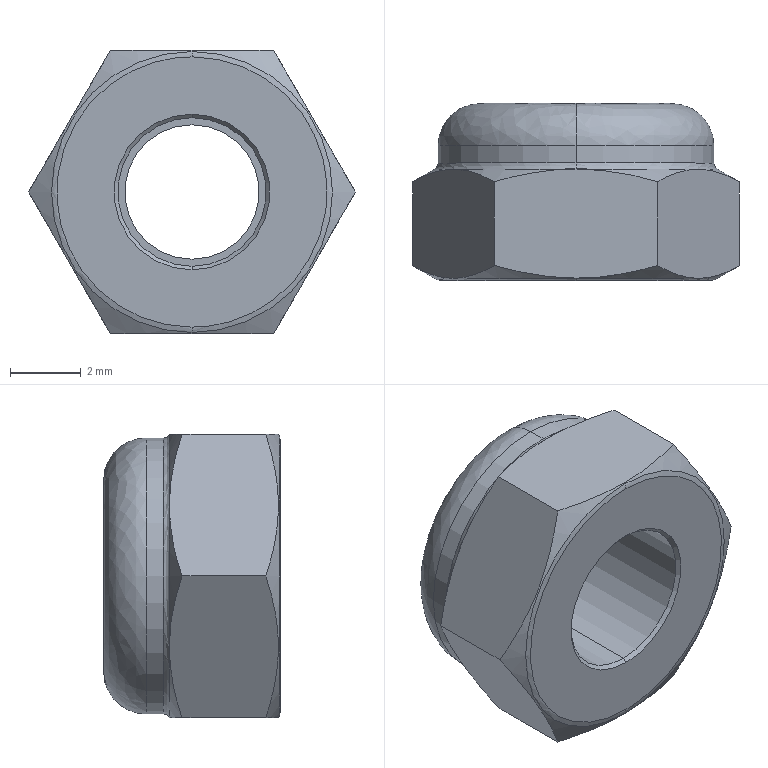Part | SolidWorks | features BaseBody 1 | 1 solid | 39 faces | box 9.238 x 5 x 8 mm | volume 186.691 mm3 | plane 11 | cone 10 | cylinder 10 | spline 8 | commonest cylinder face diameters 3.8 x2 4.2 x2 5 x2 6 x2 7.8 x2
STEP:
#1=CARTESIAN_POINT('',(0.,-1.56,3.97));
#2=VERTEX_POINT('',#1);
#3=CARTESIAN_POINT('',(0.,-1.56,-3.97));
#4=VERTEX_POINT('',#3);
#5=CARTESIAN_POINT('',(0.,-1.56,0.));
#6=DIRECTION('',(0.,-1.,0.));
#7=DIRECTION('',(0.,0.,1.));
#8=AXIS2_PLACEMENT_3D('',#5,#6,#7);
#9=CIRCLE('',#8,3.97);
#10=EDGE_CURVE('',#2,#4,#9,.T.);
#11=ORIENTED_EDGE('',*,*,#10,.T.);
#12=CARTESIAN_POINT('',(0.,-1.6,-3.82));
#13=VERTEX_POINT('',#12);
#14=CARTESIAN_POINT('',(0.,-1.3,-3.82));
#15=DIRECTION('',(-1.,0.,0.));
#16=DIRECTION('',(0.,0.,-1.));
#17=AXIS2_PLACEMENT_3D('',#14,#15,#16);
#18=CIRCLE('',#17,0.3);
#19=EDGE_CURVE('',#4,#13,#18,.T.);
#20=ORIENTED_EDGE('',*,*,#19,.T.);
#21=CARTESIAN_POINT('',(0.,-1.6,3.82));
#22=VERTEX_POINT('',#21);
#23=CARTESIAN_POINT('',(0.,-1.6,-3.82));
#24=CARTESIAN_POINT('',(-7.639,-1.6,-3.82));
#25=CARTESIAN_POINT('',(-7.639,-1.6,3.82));
#26=CARTESIAN_POINT('',(0.,-1.6,3.82));
#27=(BOUNDED_CURVE()B_SPLINE_CURVE(3,(#23,#24,#25,#26),.UNSPECIFIED.,.F.,.F.)B_SPLINE_CURVE_WITH_KNOTS((4,4),(0.,1.),.UNSPECIFIED.)CURVE()GEOMETRIC_REPRESENTATION_ITEM()RATIONAL_B_SPLINE_CURVE((1.,0.3333,0.3333,1.))REPRESENTATION_ITEM(''));
#28=EDGE_CURVE('',#13,#22,#27,.T.);
#29=ORIENTED_EDGE('',*,*,#28,.T.);
#30=CARTESIAN_POINT('',(0.,-1.3,3.82));
#31=DIRECTION('',(1.,0.,0.));
#32=DIRECTION('',(0.,0.,1.));
#33=AXIS2_PLACEMENT_3D('',#30,#31,#32);
#34=CIRCLE('',#33,0.3);
#35=EDGE_CURVE('',#2,#22,#34,.T.);
#36=ORIENTED_EDGE('',*,*,#35,.F.);
#37=EDGE_LOOP('',(#11,#20,#29,#36));
#38=FACE_OUTER_BOUND('',#37,.T.);
#39=CARTESIAN_POINT('',(0.,-1.56,-3.97));
#40=CARTESIAN_POINT('',(-7.939,-1.56,-3.97));
#41=CARTESIAN_POINT('',(-7.939,-1.56,3.97));
#42=CARTESIAN_POINT('',(0.,-1.56,3.97));
#43=CARTESIAN_POINT('',(0.,-1.586,-3.924));
#44=CARTESIAN_POINT('',(-7.847,-1.586,-3.924));
#45=CARTESIAN_POINT('',(-7.847,-1.586,3.924));
#46=CARTESIAN_POINT('',(0.,-1.586,3.924));
#47=CARTESIAN_POINT('',(0.,-1.6,-3.873));
#48=CARTESIAN_POINT('',(-7.745,-1.6,-3.873));
#49=CARTESIAN_POINT('',(-7.745,-1.6,3.873));
#50=CARTESIAN_POINT('',(0.,-1.6,3.873));
#51=CARTESIAN_POINT('',(0.,-1.6,-3.82));
#52=CARTESIAN_POINT('',(-7.639,-1.6,-3.82));
#53=CARTESIAN_POINT('',(-7.639,-1.6,3.82));
#54=CARTESIAN_POINT('',(0.,-1.6,3.82));
#55=(BOUNDED_SURFACE()B_SPLINE_SURFACE(3,3,((#39,#40,#41,#42),(#43,#44,#45,#46),(#47,#48,#49,#50),(#51,#52,#53,#54)),.UNSPECIFIED.,.F.,.F.,.F.)B_SPLINE_SURFACE_WITH_KNOTS((4,4),(4,4),(0.,1.),(0.,1.),.UNSPECIFIED.)GEOMETRIC_REPRESENTATION_ITEM()RATIONAL_B_SPLINE_SURFACE(((1.,0.3333,0.3333,1.),(0.9773,0.3258,0.3258,0.9773),(0.9773,0.3258,0.3258,0.9773),(1.,0.3333,0.3333,1.)))REPRESENTATION_ITEM('')SURFACE());
#56=ADVANCED_FACE('',(#38),#55,.T.);
#57=CARTESIAN_POINT('',(0.,1.542,-4.));
#58=VERTEX_POINT('',#57);
#59=CARTESIAN_POINT('',(3.464,1.542,-2.));
#60=VERTEX_POINT('',#59);
#61=CARTESIAN_POINT('',(0.,1.542,0.));
#62=DIRECTION('',(0.,-1.,0.));
#63=DIRECTION('',(0.,0.,-1.));
#64=AXIS2_PLACEMENT_3D('',#61,#62,#63);
#65=CIRCLE('',#64,4.);
#66=EDGE_CURVE('',#58,#60,#65,.T.);
#67=ORIENTED_EDGE('',*,*,#66,.F.);
#68=CARTESIAN_POINT('',(0.,1.715,-3.9));
#69=VERTEX_POINT('',#68);
#70=CARTESIAN_POINT('',(0.,1.715,-4.1));
#71=DIRECTION('',(-1.,0.,0.));
#72=DIRECTION('',(0.,0.,-1.));
#73=AXIS2_PLACEMENT_3D('',#70,#71,#72);
#74=CIRCLE('',#73,0.2);
#75=EDGE_CURVE('',#58,#69,#74,.T.);
#76=ORIENTED_EDGE('',*,*,#75,.T.);
#77=CARTESIAN_POINT('',(0.,1.715,3.9));
#78=VERTEX_POINT('',#77);
#79=CARTESIAN_POINT('',(0.,1.715,0.));
#80=DIRECTION('',(0.,1.,0.));
#81=DIRECTION('',(0.,0.,1.));
#82=AXIS2_PLACEMENT_3D('',#79,#80,#81);
#83=CIRCLE('',#82,3.9);
#84=EDGE_CURVE('',#78,#69,#83,.T.);
#85=ORIENTED_EDGE('',*,*,#84,.F.);
#86=CARTESIAN_POINT('',(0.,1.542,4.));
#87=VERTEX_POINT('',#86);
#88=CARTESIAN_POINT('',(0.,1.715,4.1));
#89=DIRECTION('',(1.,0.,0.));
#90=DIRECTION('',(0.,0.,1.));
#91=AXIS2_PLACEMENT_3D('',#88,#89,#90);
#92=CIRCLE('',#91,0.2);
#93=EDGE_CURVE('',#87,#78,#92,.T.);
#94=ORIENTED_EDGE('',*,*,#93,.F.);
#95=CARTESIAN_POINT('',(3.464,1.542,2.));
#96=VERTEX_POINT('',#95);
#97=CARTESIAN_POINT('',(0.,1.542,0.));
#98=DIRECTION('',(0.,-1.,0.));
#99=DIRECTION('',(0.,0.,-1.));
#100=AXIS2_PLACEMENT_3D('',#97,#98,#99);
#101=CIRCLE('',#100,4.);
#102=EDGE_CURVE('',#96,#87,#101,.T.);
#103=ORIENTED_EDGE('',*,*,#102,.F.);
#104=CARTESIAN_POINT('',(0.,1.542,0.));
#105=DIRECTION('',(0.,-1.,0.));
#106=DIRECTION('',(0.,0.,-1.));
#107=AXIS2_PLACEMENT_3D('',#104,#105,#106);
#108=CIRCLE('',#107,4.);
#109=EDGE_CURVE('',#60,#96,#108,.T.);
#110=ORIENTED_EDGE('',*,*,#109,.F.);
#111=EDGE_LOOP('',(#67,#76,#85,#94,#103,#110));
#112=FACE_OUTER_BOUND('',#111,.T.);
#113=CARTESIAN_POINT('',(0.,1.542,4.));
#114=CARTESIAN_POINT('',(8.,1.542,4.));
#115=CARTESIAN_POINT('',(8.,1.542,-4.));
#116=CARTESIAN_POINT('',(0.,1.542,-4.));
#117=CARTESIAN_POINT('',(0.,1.579,3.937));
#118=CARTESIAN_POINT('',(7.873,1.579,3.937));
#119=CARTESIAN_POINT('',(7.873,1.579,-3.937));
#120=CARTESIAN_POINT('',(0.,1.579,-3.937));
#121=CARTESIAN_POINT('',(0.,1.642,3.9));
#122=CARTESIAN_POINT('',(7.8,1.642,3.9));
#123=CARTESIAN_POINT('',(7.8,1.642,-3.9));
#124=CARTESIAN_POINT('',(0.,1.642,-3.9));
#125=CARTESIAN_POINT('',(0.,1.715,3.9));
#126=CARTESIAN_POINT('',(7.8,1.715,3.9));
#127=CARTESIAN_POINT('',(7.8,1.715,-3.9));
#128=CARTESIAN_POINT('',(0.,1.715,-3.9));
#129=(BOUNDED_SURFACE()B_SPLINE_SURFACE(3,3,((#113,#114,#115,#116),(#117,#118,#119,#120),(#121,#122,#123,#124),(#125,#126,#127,#128)),.UNSPECIFIED.,.F.,.F.,.F.)B_SPLINE_SURFACE_WITH_KNOTS((4,4),(4,4),(0.,1.),(0.,1.),.UNSPECIFIED.)GEOMETRIC_REPRESENTATION_ITEM()RATIONAL_B_SPLINE_SURFACE(((1.,0.3333,0.3333,1.),(0.9107,0.3036,0.3036,0.9107),(0.9107,0.3036,0.3036,0.9107),(1.,0.3333,0.3333,1.)))REPRESENTATION_ITEM('')SURFACE());
#130=ADVANCED_FACE('',(#112),#129,.F.);
#131=CARTESIAN_POINT('',(0.,3.4,2.7));
#132=VERTEX_POINT('',#131);
#133=CARTESIAN_POINT('',(0.,3.4,-2.7));
#134=VERTEX_POINT('',#133);
#135=CARTESIAN_POINT('',(0.,3.4,2.7));
#136=CARTESIAN_POINT('',(-5.4,3.4,2.7));
#137=CARTESIAN_POINT('',(-5.4,3.4,-2.7));
#138=CARTESIAN_POINT('',(0.,3.4,-2.7));
#139=(BOUNDED_CURVE()B_SPLINE_CURVE(3,(#135,#136,#137,#138),.UNSPECIFIED.,.F.,.F.)B_SPLINE_CURVE_WITH_KNOTS((4,4),(0.,1.),.UNSPECIFIED.)CURVE()GEOMETRIC_REPRESENTATION_ITEM()RATIONAL_B_SPLINE_CURVE((1.,0.3333,0.3333,1.))REPRESENTATION_ITEM(''));
#140=EDGE_CURVE('',#132,#134,#139,.T.);
#141=ORIENTED_EDGE('',*,*,#140,.T.);
#142=CARTESIAN_POINT('',(0.,2.2,-3.9));
#143=VERTEX_POINT('',#142);
#144=CARTESIAN_POINT('',(0.,2.2,-2.7));
#145=DIRECTION('',(-1.,0.,0.));
#146=DIRECTION('',(0.,0.,-1.));
#147=AXIS2_PLACEMENT_3D('',#144,#145,#146);
#148=CIRCLE('',#147,1.2);
#149=EDGE_CURVE('',#134,#143,#148,.T.);
#150=ORIENTED_EDGE('',*,*,#149,.T.);
#151=CARTESIAN_POINT('',(0.,2.2,3.9));
#152=VERTEX_POINT('',#151);
#153=CARTESIAN_POINT('',(0.,2.2,0.));
#154=DIRECTION('',(0.,-1.,0.));
#155=DIRECTION('',(0.,0.,1.));
#156=AXIS2_PLACEMENT_3D('',#153,#154,#155);
#157=CIRCLE('',#156,3.9);
#158=EDGE_CURVE('',#152,#143,#157,.T.);
#159=ORIENTED_EDGE('',*,*,#158,.F.);
#160=CARTESIAN_POINT('',(0.,2.2,2.7));
#161=DIRECTION('',(1.,0.,0.));
#162=DIRECTION('',(0.,0.,1.));
#163=AXIS2_PLACEMENT_3D('',#160,#161,#162);
#164=CIRCLE('',#163,1.2);
#165=EDGE_CURVE('',#132,#152,#164,.T.);
#166=ORIENTED_EDGE('',*,*,#165,.F.);
#167=EDGE_LOOP('',(#141,#150,#159,#166));
#168=FACE_OUTER_BOUND('',#167,.T.);
#169=CARTESIAN_POINT('',(0.,3.4,-2.7));
#170=CARTESIAN_POINT('',(-5.4,3.4,-2.7));
#171=CARTESIAN_POINT('',(-5.4,3.4,2.7));
#172=CARTESIAN_POINT('',(0.,3.4,2.7));
#173=CARTESIAN_POINT('',(0.,3.4,-3.403));
#174=CARTESIAN_POINT('',(-6.806,3.4,-3.403));
#175=CARTESIAN_POINT('',(-6.806,3.4,3.403));
#176=CARTESIAN_POINT('',(0.,3.4,3.403));
#177=CARTESIAN_POINT('',(0.,2.903,-3.9));
#178=CARTESIAN_POINT('',(-7.8,2.903,-3.9));
#179=CARTESIAN_POINT('',(-7.8,2.903,3.9));
#180=CARTESIAN_POINT('',(0.,2.903,3.9));
#181=CARTESIAN_POINT('',(0.,2.2,-3.9));
#182=CARTESIAN_POINT('',(-7.8,2.2,-3.9));
#183=CARTESIAN_POINT('',(-7.8,2.2,3.9));
#184=CARTESIAN_POINT('',(0.,2.2,3.9));
#185=(BOUNDED_SURFACE()B_SPLINE_SURFACE(3,3,((#169,#170,#171,#172),(#173,#174,#175,#176),(#177,#178,#179,#180),(#181,#182,#183,#184)),.UNSPECIFIED.,.F.,.F.,.F.)B_SPLINE_SURFACE_WITH_KNOTS((4,4),(4,4),(0.,1.),(0.,1.),.UNSPECIFIED.)GEOMETRIC_REPRESENTATION_ITEM()RATIONAL_B_SPLINE_SURFACE(((1.,0.3333,0.3333,1.),(0.8047,0.2682,0.2682,0.8047),(0.8047,0.2682,0.2682,0.8047),(1.,0.3333,0.3333,1.)))REPRESENTATION_ITEM('')SURFACE());
#186=ADVANCED_FACE('',(#168),#185,.T.);
#187=CARTESIAN_POINT('',(0.,3.25,2.5));
#188=VERTEX_POINT('',#187);
#189=CARTESIAN_POINT('',(0.,3.25,-2.5));
#190=VERTEX_POINT('',#189);
#191=CARTESIAN_POINT('',(0.,3.25,0.));
#192=DIRECTION('',(0.,-1.,0.));
#193=DIRECTION('',(0.,0.,1.));
#194=AXIS2_PLACEMENT_3D('',#191,#192,#193);
#195=CIRCLE('',#194,2.5);
#196=EDGE_CURVE('',#188,#190,#195,.T.);
#197=ORIENTED_EDGE('',*,*,#196,.T.);
#198=CARTESIAN_POINT('',(0.,3.4,-2.65));
#199=VERTEX_POINT('',#198);
#200=CARTESIAN_POINT('',(0.,3.25,-2.65));
#201=DIRECTION('',(-1.,0.,0.));
#202=DIRECTION('',(0.,0.,-1.));
#203=AXIS2_PLACEMENT_3D('',#200,#201,#202);
#204=CIRCLE('',#203,0.15);
#205=EDGE_CURVE('',#190,#199,#204,.T.);
#206=ORIENTED_EDGE('',*,*,#205,.T.);
#207=CARTESIAN_POINT('',(0.,3.4,2.65));
#208=VERTEX_POINT('',#207);
#209=CARTESIAN_POINT('',(0.,3.4,2.65));
#210=CARTESIAN_POINT('',(-0.1684,3.4,2.65));
#211=CARTESIAN_POINT('',(-0.4166,3.4,2.627));
#212=CARTESIAN_POINT('',(-0.6986,3.4,2.559));
#213=CARTESIAN_POINT('',(-0.8377,3.4,2.515));
#214=CARTESIAN_POINT('',(-0.8968,3.4,2.494));
#215=CARTESIAN_POINT('',(-0.9362,3.4,2.479));
#216=CARTESIAN_POINT('',(-0.9542,3.4,2.472));
#217=CARTESIAN_POINT('',(-1.315,3.4,2.329));
#218=CARTESIAN_POINT('',(-1.615,3.4,2.132));
#219=CARTESIAN_POINT('',(-2.003,3.4,1.745));
#220=CARTESIAN_POINT('',(-2.174,3.4,1.535));
#221=CARTESIAN_POINT('',(-2.332,3.4,1.264));
#222=CARTESIAN_POINT('',(-2.402,3.4,1.122));
#223=CARTESIAN_POINT('',(-2.429,3.4,1.06));
#224=CARTESIAN_POINT('',(-2.447,3.4,1.018));
#225=CARTESIAN_POINT('',(-2.456,3.4,0.995));
#226=CARTESIAN_POINT('',(-2.588,3.4,0.6625));
#227=CARTESIAN_POINT('',(-2.65,3.4,0.3366));
#228=CARTESIAN_POINT('',(-2.65,3.4,-0.1683));
#229=CARTESIAN_POINT('',(-2.627,3.4,-0.4165));
#230=CARTESIAN_POINT('',(-2.559,3.4,-0.6985));
#231=CARTESIAN_POINT('',(-2.515,3.4,-0.8376));
#232=CARTESIAN_POINT('',(-2.494,3.4,-0.8968));
#233=CARTESIAN_POINT('',(-2.479,3.4,-0.9362));
#234=CARTESIAN_POINT('',(-2.472,3.4,-0.9542));
#235=CARTESIAN_POINT('',(-2.329,3.4,-1.315));
#236=CARTESIAN_POINT('',(-2.132,3.4,-1.615));
#237=CARTESIAN_POINT('',(-1.745,3.4,-2.003));
#238=CARTESIAN_POINT('',(-1.535,3.4,-2.174));
#239=CARTESIAN_POINT('',(-1.264,3.4,-2.332));
#240=CARTESIAN_POINT('',(-1.122,3.4,-2.402));
#241=CARTESIAN_POINT('',(-1.06,3.4,-2.429));
#242=CARTESIAN_POINT('',(-1.018,3.4,-2.447));
#243=CARTESIAN_POINT('',(-0.995,3.4,-2.456));
#244=CARTESIAN_POINT('',(-0.6623,3.4,-2.588));
#245=CARTESIAN_POINT('',(-0.3372,3.4,-2.65));
#246=CARTESIAN_POINT('',(0.,3.4,-2.65));
#247=B_SPLINE_CURVE_WITH_KNOTS('',3,(#209,#210,#211,#212,#213,#214,#215,#216,#217,#218,#219,#220,#221,#222,#223,#224,#225,#226,#227,#228,#229,#230,#231,#232,#233,#234,#235,#236,#237,#238,#239,#240,#241,#242,#243,#244,#245,#246),.UNSPECIFIED.,.F.,.F.,(4,1,1,1,2,2,2,1,1,1,2,2,2,1,1,1,2,2,2,1,1,1,2,2,4),(0.,0.0625,0.09375,0.1094,0.1172,0.125,0.25,0.3125,0.3437,0.3594,0.3672,0.375,0.5,0.5625,0.5937,0.6094,0.6172,0.625,0.75,0.8125,0.8437,0.8594,0.8672,0.875,1.),.UNSPECIFIED.);
#248=EDGE_CURVE('',#208,#199,#247,.T.);
#249=ORIENTED_EDGE('',*,*,#248,.F.);
#250=CARTESIAN_POINT('',(0.,3.25,2.65));
#251=DIRECTION('',(1.,0.,0.));
#252=DIRECTION('',(0.,0.,1.));
#253=AXIS2_PLACEMENT_3D('',#250,#251,#252);
#254=CIRCLE('',#253,0.15);
#255=EDGE_CURVE('',#188,#208,#254,.T.);
#256=ORIENTED_EDGE('',*,*,#255,.F.);
#257=EDGE_LOOP('',(#197,#206,#249,#256));
#258=FACE_OUTER_BOUND('',#257,.T.);
#259=CARTESIAN_POINT('',(0.,3.25,-2.5));
#260=CARTESIAN_POINT('',(-5.,3.25,-2.5));
#261=CARTESIAN_POINT('',(-5.,3.25,2.5));
#262=CARTESIAN_POINT('',(0.,3.25,2.5));
#263=CARTESIAN_POINT('',(0.,3.338,-2.5));
#264=CARTESIAN_POINT('',(-5.,3.338,-2.5));
#265=CARTESIAN_POINT('',(-5.,3.338,2.5));
#266=CARTESIAN_POINT('',(0.,3.338,2.5));
#267=CARTESIAN_POINT('',(0.,3.4,-2.562));
#268=CARTESIAN_POINT('',(-5.124,3.4,-2.562));
#269=CARTESIAN_POINT('',(-5.124,3.4,2.562));
#270=CARTESIAN_POINT('',(0.,3.4,2.562));
#271=CARTESIAN_POINT('',(0.,3.4,-2.65));
#272=CARTESIAN_POINT('',(-5.3,3.4,-2.65));
#273=CARTESIAN_POINT('',(-5.3,3.4,2.65));
#274=CARTESIAN_POINT('',(0.,3.4,2.65));
#275=(BOUNDED_SURFACE()B_SPLINE_SURFACE(3,3,((#259,#260,#261,#262),(#263,#264,#265,#266),(#267,#268,#269,#270),(#271,#272,#273,#274)),.UNSPECIFIED.,.F.,.F.,.F.)B_SPLINE_SURFACE_WITH_KNOTS((4,4),(4,4),(0.,1.),(0.,1.),.UNSPECIFIED.)GEOMETRIC_REPRESENTATION_ITEM()RATIONAL_B_SPLINE_SURFACE(((1.,0.3333,0.3333,1.),(0.8047,0.2682,0.2682,0.8047),(0.8047,0.2682,0.2682,0.8047),(1.,0.3333,0.3333,1.)))REPRESENTATION_ITEM('')SURFACE());
#276=ADVANCED_FACE('',(#258),#275,.T.);
#277=CARTESIAN_POINT('',(0.,-1.5,2.1));
#278=VERTEX_POINT('',#277);
#279=CARTESIAN_POINT('',(0.,-1.5,-2.1));
#280=VERTEX_POINT('',#279);
#281=CARTESIAN_POINT('',(0.,-1.5,0.));
#282=DIRECTION('',(0.,-1.,0.));
#283=DIRECTION('',(0.,0.,-1.));
#284=AXIS2_PLACEMENT_3D('',#281,#282,#283);
#285=CIRCLE('',#284,2.1);
#286=EDGE_CURVE('',#278,#280,#285,.T.);
#287=ORIENTED_EDGE('',*,*,#286,.F.);
#288=CARTESIAN_POINT('',(0.,-1.6,2.2));
#289=VERTEX_POINT('',#288);
#290=CARTESIAN_POINT('',(0.,-1.6,2.2));
#291=DIRECTION('',(0.,-0.7071,0.7071));
#292=VECTOR('',#291,1000.);
#293=LINE('',#290,#292);
#294=EDGE_CURVE('',#278,#289,#293,.T.);
#295=ORIENTED_EDGE('',*,*,#294,.T.);
#296=CARTESIAN_POINT('',(0.,-1.6,-2.2));
#297=VERTEX_POINT('',#296);
#298=CARTESIAN_POINT('',(0.,-1.6,0.));
#299=DIRECTION('',(0.,-1.,0.));
#300=DIRECTION('',(0.,0.,-1.));
#301=AXIS2_PLACEMENT_3D('',#298,#299,#300);
#302=CIRCLE('',#301,2.2);
#303=EDGE_CURVE('',#289,#297,#302,.T.);
#304=ORIENTED_EDGE('',*,*,#303,.T.);
#305=CARTESIAN_POINT('',(0.,-1.6,-2.2));
#306=DIRECTION('',(0.,-0.7071,-0.7071));
#307=VECTOR('',#306,1000.);
#308=LINE('',#305,#307);
#309=EDGE_CURVE('',#280,#297,#308,.T.);
#310=ORIENTED_EDGE('',*,*,#309,.F.);
#311=EDGE_LOOP('',(#287,#295,#304,#310));
#312=FACE_OUTER_BOUND('',#311,.T.);
#313=CARTESIAN_POINT('',(0.,-1.6,0.));
#314=DIRECTION('',(0.,-1.,0.));
#315=DIRECTION('',(0.,0.,-1.));
#316=AXIS2_PLACEMENT_3D('',#313,#314,#315);
#317=CONICAL_SURFACE('',#316,2.2,0.7854);
#318=ADVANCED_FACE('',(#312),#317,.F.);
#319=CARTESIAN_POINT('',(0.,-1.56,0.));
#320=DIRECTION('',(0.,-1.,0.));
#321=DIRECTION('',(0.,0.,1.));
#322=AXIS2_PLACEMENT_3D('',#319,#320,#321);
#323=CIRCLE('',#322,3.97);
#324=EDGE_CURVE('',#4,#2,#323,.T.);
#325=ORIENTED_EDGE('',*,*,#324,.F.);
#326=CARTESIAN_POINT('',(0.,-1.542,-4.));
#327=VERTEX_POINT('',#326);
#328=CARTESIAN_POINT('',(0.,-1.183,-4.623));
#329=DIRECTION('',(0.,0.5,-0.866));
#330=VECTOR('',#329,1000.);
#331=LINE('',#328,#330);
#332=EDGE_CURVE('',#4,#327,#331,.T.);
#333=ORIENTED_EDGE('',*,*,#332,.T.);
#334=CARTESIAN_POINT('',(2.309,-1.185,-4.));
#335=VERTEX_POINT('',#334);
#336=CARTESIAN_POINT('',(0.,-1.542,-4.));
#337=CARTESIAN_POINT('',(0.7882,-1.542,-4.));
#338=CARTESIAN_POINT('',(1.555,-1.403,-4.));
#339=CARTESIAN_POINT('',(2.309,-1.185,-4.));
#340=B_SPLINE_CURVE_WITH_KNOTS('',3,(#336,#337,#338,#339),.UNSPECIFIED.,.F.,.F.,(4,4),(0.002337,0.004674),.UNSPECIFIED.);
#341=EDGE_CURVE('',#327,#335,#340,.T.);
#342=ORIENTED_EDGE('',*,*,#341,.T.);
#343=CARTESIAN_POINT('',(4.619,-1.185,-0.000000043));
#344=VERTEX_POINT('',#343);
#345=CARTESIAN_POINT('',(2.309,-1.185,-4.));
#346=CARTESIAN_POINT('',(2.686,-1.403,-3.347));
#347=CARTESIAN_POINT('',(3.069,-1.542,-2.684));
#348=CARTESIAN_POINT('',(3.658,-1.543,-1.664));
#349=CARTESIAN_POINT('',(3.854,-1.508,-1.324));
#350=CARTESIAN_POINT('',(4.24,-1.384,-0.6567));
#351=CARTESIAN_POINT('',(4.43,-1.294,-0.327));
#352=CARTESIAN_POINT('',(4.619,-1.185,-0.000000043));
#353=B_SPLINE_CURVE_WITH_KNOTS('',3,(#345,#346,#347,#348,#349,#350,#351,#352),.UNSPECIFIED.,.F.,.F.,(4,2,2,4),(0.,0.002332,0.003499,0.004665),.UNSPECIFIED.);
#354=EDGE_CURVE('',#335,#344,#353,.T.);
#355=ORIENTED_EDGE('',*,*,#354,.T.);
#356=CARTESIAN_POINT('',(2.309,-1.185,4.));
#357=VERTEX_POINT('',#356);
#358=CARTESIAN_POINT('',(4.619,-1.185,-0.000000043));
#359=CARTESIAN_POINT('',(4.242,-1.403,0.6531));
#360=CARTESIAN_POINT('',(3.859,-1.542,1.316));
#361=CARTESIAN_POINT('',(3.27,-1.543,2.336));
#362=CARTESIAN_POINT('',(3.074,-1.508,2.676));
#363=CARTESIAN_POINT('',(2.689,-1.384,3.343));
#364=CARTESIAN_POINT('',(2.498,-1.294,3.673));
#365=CARTESIAN_POINT('',(2.309,-1.185,4.));
#366=B_SPLINE_CURVE_WITH_KNOTS('',3,(#358,#359,#360,#361,#362,#363,#364,#365),.UNSPECIFIED.,.F.,.F.,(4,2,2,4),(0.,0.002332,0.003499,0.004665),.UNSPECIFIED.);
#367=EDGE_CURVE('',#344,#357,#366,.T.);
#368=ORIENTED_EDGE('',*,*,#367,.T.);
#369=CARTESIAN_POINT('',(0.,-1.542,4.));
#370=VERTEX_POINT('',#369);
#371=CARTESIAN_POINT('',(2.309,-1.185,4.));
#372=CARTESIAN_POINT('',(1.555,-1.403,4.));
#373=CARTESIAN_POINT('',(0.7882,-1.542,4.));
#374=CARTESIAN_POINT('',(0.,-1.542,4.));
#375=B_SPLINE_CURVE_WITH_KNOTS('',3,(#371,#372,#373,#374),.UNSPECIFIED.,.F.,.F.,(4,4),(-0.002337,0.),.UNSPECIFIED.);
#376=EDGE_CURVE('',#357,#370,#375,.T.);
#377=ORIENTED_EDGE('',*,*,#376,.T.);
#378=CARTESIAN_POINT('',(0.,-1.183,4.623));
#379=DIRECTION('',(0.,0.5,0.866));
#380=VECTOR('',#379,1000.);
#381=LINE('',#378,#380);
#382=EDGE_CURVE('',#2,#370,#381,.T.);
#383=ORIENTED_EDGE('',*,*,#382,.F.);
#384=EDGE_LOOP('',(#325,#333,#342,#355,#368,#377,#383));
#385=FACE_OUTER_BOUND('',#384,.T.);
#386=CARTESIAN_POINT('',(0.,-1.183,0.));
#387=DIRECTION('',(0.,1.,0.));
#388=DIRECTION('',(0.,0.,1.));
#389=AXIS2_PLACEMENT_3D('',#386,#387,#388);
#390=CONICAL_SURFACE('',#389,4.623,1.047);
#391=ADVANCED_FACE('',(#385),#390,.T.);
#392=CARTESIAN_POINT('',(0.,1.6,2.1));
#393=VERTEX_POINT('',#392);
#394=CARTESIAN_POINT('',(0.,1.6,-2.1));
#395=VERTEX_POINT('',#394);
#396=CARTESIAN_POINT('',(0.,1.6,0.));
#397=DIRECTION('',(0.,-1.,0.));
#398=DIRECTION('',(0.,0.,-1.));
#399=AXIS2_PLACEMENT_3D('',#396,#397,#398);
#400=CIRCLE('',#399,2.1);
#401=EDGE_CURVE('',#393,#395,#400,.T.);
#402=ORIENTED_EDGE('',*,*,#401,.F.);
#403=CARTESIAN_POINT('',(0.,1.6,2.1));
#404=DIRECTION('',(0.,-1.,0.));
#405=VECTOR('',#404,1000.);
#406=LINE('',#403,#405);
#407=EDGE_CURVE('',#393,#278,#406,.T.);
#408=ORIENTED_EDGE('',*,*,#407,.T.);
#409=ORIENTED_EDGE('',*,*,#286,.T.);
#410=CARTESIAN_POINT('',(0.,1.6,-2.1));
#411=DIRECTION('',(0.,-1.,0.));
#412=VECTOR('',#411,1000.);
#413=LINE('',#410,#412);
#414=EDGE_CURVE('',#395,#280,#413,.T.);
#415=ORIENTED_EDGE('',*,*,#414,.F.);
#416=EDGE_LOOP('',(#402,#408,#409,#415));
#417=FACE_OUTER_BOUND('',#416,.T.);
#418=CARTESIAN_POINT('',(0.,1.6,0.));
#419=DIRECTION('',(0.,-1.,0.));
#420=DIRECTION('',(0.,0.,-1.));
#421=AXIS2_PLACEMENT_3D('',#418,#419,#420);
#422=CYLINDRICAL_SURFACE('',#421,2.1);
#423=ADVANCED_FACE('',(#417),#422,.F.);
#424=CARTESIAN_POINT('',(0.,1.6,-1.9));
#425=VERTEX_POINT('',#424);
#426=CARTESIAN_POINT('',(0.,1.6,1.9));
#427=VERTEX_POINT('',#426);
#428=CARTESIAN_POINT('',(0.,1.6,0.));
#429=DIRECTION('',(0.,1.,0.));
#430=DIRECTION('',(0.,0.,1.));
#431=AXIS2_PLACEMENT_3D('',#428,#429,#430);
#432=CIRCLE('',#431,1.9);
#433=EDGE_CURVE('',#425,#427,#432,.T.);
#434=ORIENTED_EDGE('',*,*,#433,.F.);
#435=CARTESIAN_POINT('',(0.,3.057,-1.9));
#436=VERTEX_POINT('',#435);
#437=CARTESIAN_POINT('',(0.,2.514,-1.9));
#438=DIRECTION('',(0.,1.,0.));
#439=VECTOR('',#438,1000.);
#440=LINE('',#437,#439);
#441=EDGE_CURVE('',#425,#436,#440,.T.);
#442=ORIENTED_EDGE('',*,*,#441,.T.);
#443=CARTESIAN_POINT('',(0.,3.057,1.9));
#444=VERTEX_POINT('',#443);
#445=CARTESIAN_POINT('',(0.,3.057,0.));
#446=DIRECTION('',(0.,-1.,0.));
#447=DIRECTION('',(0.,0.,1.));
#448=AXIS2_PLACEMENT_3D('',#445,#446,#447);
#449=CIRCLE('',#448,1.9);
#450=EDGE_CURVE('',#444,#436,#449,.T.);
#451=ORIENTED_EDGE('',*,*,#450,.F.);
#452=CARTESIAN_POINT('',(0.,2.514,1.9));
#453=DIRECTION('',(0.,1.,0.));
#454=VECTOR('',#453,1000.);
#455=LINE('',#452,#454);
#456=EDGE_CURVE('',#427,#444,#455,.T.);
#457=ORIENTED_EDGE('',*,*,#456,.F.);
#458=EDGE_LOOP('',(#434,#442,#451,#457));
#459=FACE_OUTER_BOUND('',#458,.T.);
#460=CARTESIAN_POINT('',(0.,2.514,0.));
#461=DIRECTION('',(0.,1.,0.));
#462=DIRECTION('',(0.,0.,1.));
#463=AXIS2_PLACEMENT_3D('',#460,#461,#462);
#464=CYLINDRICAL_SURFACE('',#463,1.9);
#465=ADVANCED_FACE('',(#459),#464,.F.);
#466=ORIENTED_EDGE('',*,*,#84,.T.);
#467=CARTESIAN_POINT('',(0.,2.805,-3.9));
#468=DIRECTION('',(0.,1.,0.));
#469=VECTOR('',#468,1000.);
#470=LINE('',#467,#469);
#471=EDGE_CURVE('',#69,#143,#470,.T.);
#472=ORIENTED_EDGE('',*,*,#471,.T.);
#473=CARTESIAN_POINT('',(0.,2.2,0.));
#474=DIRECTION('',(0.,-1.,0.));
#475=DIRECTION('',(0.,0.,1.));
#476=AXIS2_PLACEMENT_3D('',#473,#474,#475);
#477=CIRCLE('',#476,3.9);
#478=EDGE_CURVE('',#143,#152,#477,.T.);
#479=ORIENTED_EDGE('',*,*,#478,.T.);
#480=CARTESIAN_POINT('',(0.,2.805,3.9));
#481=DIRECTION('',(0.,1.,0.));
#482=VECTOR('',#481,1000.);
#483=LINE('',#480,#482);
#484=EDGE_CURVE('',#78,#152,#483,.T.);
#485=ORIENTED_EDGE('',*,*,#484,.F.);
#486=EDGE_LOOP('',(#466,#472,#479,#485));
#487=FACE_OUTER_BOUND('',#486,.T.);
#488=CARTESIAN_POINT('',(0.,2.805,0.));
#489=DIRECTION('',(0.,1.,0.));
#490=DIRECTION('',(0.,0.,1.));
#491=AXIS2_PLACEMENT_3D('',#488,#489,#490);
#492=CYLINDRICAL_SURFACE('',#491,3.9);
#493=ADVANCED_FACE('',(#487),#492,.T.);
#494=CARTESIAN_POINT('',(0.,3.057,-3.));
#495=VERTEX_POINT('',#494);
#496=CARTESIAN_POINT('',(0.,3.057,3.));
#497=VERTEX_POINT('',#496);
#498=CARTESIAN_POINT('',(0.,3.057,0.));
#499=DIRECTION('',(0.,1.,0.));
#500=DIRECTION('',(0.,0.,1.));
#501=AXIS2_PLACEMENT_3D('',#498,#499,#500);
#502=CIRCLE('',#501,3.);
#503=EDGE_CURVE('',#495,#497,#502,.T.);
#504=ORIENTED_EDGE('',*,*,#503,.F.);
#505=CARTESIAN_POINT('',(0.,3.067,-3.));
#506=VERTEX_POINT('',#505);
#507=CARTESIAN_POINT('',(0.,2.805,-3.));
#508=DIRECTION('',(0.,1.,0.));
#509=VECTOR('',#508,1000.);
#510=LINE('',#507,#509);
#511=EDGE_CURVE('',#495,#506,#510,.T.);
#512=ORIENTED_EDGE('',*,*,#511,.T.);
#513=CARTESIAN_POINT('',(0.,3.067,3.));
#514=VERTEX_POINT('',#513);
#515=CARTESIAN_POINT('',(0.,3.067,0.));
#516=DIRECTION('',(0.,-1.,0.));
#517=DIRECTION('',(0.,0.,1.));
#518=AXIS2_PLACEMENT_3D('',#515,#516,#517);
#519=CIRCLE('',#518,3.);
#520=EDGE_CURVE('',#514,#506,#519,.T.);
#521=ORIENTED_EDGE('',*,*,#520,.F.);
#522=CARTESIAN_POINT('',(0.,2.805,3.));
#523=DIRECTION('',(0.,1.,0.));
#524=VECTOR('',#523,1000.);
#525=LINE('',#522,#524);
#526=EDGE_CURVE('',#497,#514,#525,.T.);
#527=ORIENTED_EDGE('',*,*,#526,.F.);
#528=EDGE_LOOP('',(#504,#512,#521,#527));
#529=FACE_OUTER_BOUND('',#528,.T.);
#530=CARTESIAN_POINT('',(0.,2.805,0.));
#531=DIRECTION('',(0.,1.,0.));
#532=DIRECTION('',(0.,0.,1.));
#533=AXIS2_PLACEMENT_3D('',#530,#531,#532);
#534=CYLINDRICAL_SURFACE('',#533,3.);
#535=ADVANCED_FACE('',(#529),#534,.F.);
#536=CARTESIAN_POINT('',(0.,3.067,-2.5));
#537=VERTEX_POINT('',#536);
#538=CARTESIAN_POINT('',(0.,3.067,2.5));
#539=VERTEX_POINT('',#538);
#540=CARTESIAN_POINT('',(0.,3.067,0.));
#541=DIRECTION('',(0.,1.,0.));
#542=DIRECTION('',(0.,0.,1.));
#543=AXIS2_PLACEMENT_3D('',#540,#541,#542);
#544=CIRCLE('',#543,2.5);
#545=EDGE_CURVE('',#537,#539,#544,.T.);
#546=ORIENTED_EDGE('',*,*,#545,.F.);
#547=CARTESIAN_POINT('',(0.,2.805,-2.5));
#548=DIRECTION('',(0.,1.,0.));
#549=VECTOR('',#548,1000.);
#550=LINE('',#547,#549);
#551=EDGE_CURVE('',#537,#190,#550,.T.);
#552=ORIENTED_EDGE('',*,*,#551,.T.);
#553=ORIENTED_EDGE('',*,*,#196,.F.);
#554=CARTESIAN_POINT('',(0.,2.805,2.5));
#555=DIRECTION('',(0.,1.,0.));
#556=VECTOR('',#555,1000.);
#557=LINE('',#554,#556);
#558=EDGE_CURVE('',#539,#188,#557,.T.);
#559=ORIENTED_EDGE('',*,*,#558,.F.);
#560=EDGE_LOOP('',(#546,#552,#553,#559));
#561=FACE_OUTER_BOUND('',#560,.T.);
#562=CARTESIAN_POINT('',(0.,2.805,0.));
#563=DIRECTION('',(0.,1.,0.));
#564=DIRECTION('',(0.,0.,1.));
#565=AXIS2_PLACEMENT_3D('',#562,#563,#564);
#566=CYLINDRICAL_SURFACE('',#565,2.5);
#567=ADVANCED_FACE('',(#561),#566,.F.);
#568=CARTESIAN_POINT('',(0.,-1.6,3.82));
#569=CARTESIAN_POINT('',(7.639,-1.6,3.82));
#570=CARTESIAN_POINT('',(7.639,-1.6,-3.82));
#571=CARTESIAN_POINT('',(0.,-1.6,-3.82));
#572=(BOUNDED_CURVE()B_SPLINE_CURVE(3,(#568,#569,#570,#571),.UNSPECIFIED.,.F.,.F.)B_SPLINE_CURVE_WITH_KNOTS((4,4),(0.,1.),.UNSPECIFIED.)CURVE()GEOMETRIC_REPRESENTATION_ITEM()RATIONAL_B_SPLINE_CURVE((1.,0.3333,0.3333,1.))REPRESENTATION_ITEM(''));
#573=EDGE_CURVE('',#22,#13,#572,.T.);
#574=ORIENTED_EDGE('',*,*,#573,.F.);
#575=ORIENTED_EDGE('',*,*,#28,.F.);
#576=EDGE_LOOP('',(#574,#575));
#577=FACE_OUTER_BOUND('',#576,.T.);
#578=CARTESIAN_POINT('',(0.,-1.6,0.));
#579=DIRECTION('',(0.,-1.,0.));
#580=DIRECTION('',(0.,0.,-1.));
#581=AXIS2_PLACEMENT_3D('',#578,#579,#580);
#582=CIRCLE('',#581,2.2);
#583=EDGE_CURVE('',#297,#289,#582,.T.);
#584=ORIENTED_EDGE('',*,*,#583,.F.);
#585=ORIENTED_EDGE('',*,*,#303,.F.);
#586=EDGE_LOOP('',(#584,#585));
#587=FACE_BOUND('',#586,.T.);
#588=CARTESIAN_POINT('',(0.,-1.6,0.));
#589=DIRECTION('',(0.,1.,0.));
#590=DIRECTION('',(0.,0.,1.));
#591=AXIS2_PLACEMENT_3D('',#588,#589,#590);
#592=PLANE('',#591);
#593=ADVANCED_FACE('',(#577,#587),#592,.F.);
#594=ORIENTED_EDGE('',*,*,#19,.F.);
#595=ORIENTED_EDGE('',*,*,#324,.T.);
#596=ORIENTED_EDGE('',*,*,#35,.T.);
#597=ORIENTED_EDGE('',*,*,#573,.T.);
#598=EDGE_LOOP('',(#594,#595,#596,#597));
#599=FACE_OUTER_BOUND('',#598,.T.);
#600=CARTESIAN_POINT('',(0.,-1.56,3.97));
#601=CARTESIAN_POINT('',(7.939,-1.56,3.97));
#602=CARTESIAN_POINT('',(7.939,-1.56,-3.97));
#603=CARTESIAN_POINT('',(0.,-1.56,-3.97));
#604=CARTESIAN_POINT('',(0.,-1.586,3.924));
#605=CARTESIAN_POINT('',(7.847,-1.586,3.924));
#606=CARTESIAN_POINT('',(7.847,-1.586,-3.924));
#607=CARTESIAN_POINT('',(0.,-1.586,-3.924));
#608=CARTESIAN_POINT('',(0.,-1.6,3.873));
#609=CARTESIAN_POINT('',(7.745,-1.6,3.873));
#610=CARTESIAN_POINT('',(7.745,-1.6,-3.873));
#611=CARTESIAN_POINT('',(0.,-1.6,-3.873));
#612=CARTESIAN_POINT('',(0.,-1.6,3.82));
#613=CARTESIAN_POINT('',(7.639,-1.6,3.82));
#614=CARTESIAN_POINT('',(7.639,-1.6,-3.82));
#615=CARTESIAN_POINT('',(0.,-1.6,-3.82));
#616=(BOUNDED_SURFACE()B_SPLINE_SURFACE(3,3,((#600,#601,#602,#603),(#604,#605,#606,#607),(#608,#609,#610,#611),(#612,#613,#614,#615)),.UNSPECIFIED.,.F.,.F.,.F.)B_SPLINE_SURFACE_WITH_KNOTS((4,4),(4,4),(0.,1.),(0.,1.),.UNSPECIFIED.)GEOMETRIC_REPRESENTATION_ITEM()RATIONAL_B_SPLINE_SURFACE(((1.,0.3333,0.3333,1.),(0.9773,0.3258,0.3258,0.9773),(0.9773,0.3258,0.3258,0.9773),(1.,0.3333,0.3333,1.)))REPRESENTATION_ITEM('')SURFACE());
#617=ADVANCED_FACE('',(#599),#616,.T.);
#618=ORIENTED_EDGE('',*,*,#294,.F.);
#619=CARTESIAN_POINT('',(0.,-1.5,0.));
#620=DIRECTION('',(0.,-1.,0.));
#621=DIRECTION('',(0.,0.,-1.));
#622=AXIS2_PLACEMENT_3D('',#619,#620,#621);
#623=CIRCLE('',#622,2.1);
#624=EDGE_CURVE('',#280,#278,#623,.T.);
#625=ORIENTED_EDGE('',*,*,#624,.F.);
#626=ORIENTED_EDGE('',*,*,#309,.T.);
#627=ORIENTED_EDGE('',*,*,#583,.T.);
#628=EDGE_LOOP('',(#618,#625,#626,#627));
#629=FACE_OUTER_BOUND('',#628,.T.);
#630=CARTESIAN_POINT('',(0.,-1.6,0.));
#631=DIRECTION('',(0.,-1.,0.));
#632=DIRECTION('',(0.,0.,-1.));
#633=AXIS2_PLACEMENT_3D('',#630,#631,#632);
#634=CONICAL_SURFACE('',#633,2.2,0.7854);
#635=ADVANCED_FACE('',(#629),#634,.F.);
#636=ORIENTED_EDGE('',*,*,#332,.F.);
#637=ORIENTED_EDGE('',*,*,#10,.F.);
#638=ORIENTED_EDGE('',*,*,#382,.T.);
#639=CARTESIAN_POINT('',(-2.309,-1.185,4.));
#640=VERTEX_POINT('',#639);
#641=CARTESIAN_POINT('',(0.,-1.542,4.));
#642=CARTESIAN_POINT('',(-0.7882,-1.542,4.));
#643=CARTESIAN_POINT('',(-1.555,-1.403,4.));
#644=CARTESIAN_POINT('',(-2.309,-1.185,4.));
#645=B_SPLINE_CURVE_WITH_KNOTS('',3,(#641,#642,#643,#644),.UNSPECIFIED.,.F.,.F.,(4,4),(0.,0.002337),.UNSPECIFIED.);
#646=EDGE_CURVE('',#370,#640,#645,.T.);
#647=ORIENTED_EDGE('',*,*,#646,.T.);
#648=CARTESIAN_POINT('',(-4.619,-1.185,0.000000043));
#649=VERTEX_POINT('',#648);
#650=CARTESIAN_POINT('',(-2.309,-1.185,4.));
#651=CARTESIAN_POINT('',(-2.686,-1.403,3.347));
#652=CARTESIAN_POINT('',(-3.069,-1.542,2.684));
#653=CARTESIAN_POINT('',(-3.658,-1.543,1.664));
#654=CARTESIAN_POINT('',(-3.854,-1.508,1.324));
#655=CARTESIAN_POINT('',(-4.24,-1.384,0.6567));
#656=CARTESIAN_POINT('',(-4.43,-1.294,0.327));
#657=CARTESIAN_POINT('',(-4.619,-1.185,0.000000043));
#658=B_SPLINE_CURVE_WITH_KNOTS('',3,(#650,#651,#652,#653,#654,#655,#656,#657),.UNSPECIFIED.,.F.,.F.,(4,2,2,4),(0.,0.002332,0.003499,0.004665),.UNSPECIFIED.);
#659=EDGE_CURVE('',#640,#649,#658,.T.);
#660=ORIENTED_EDGE('',*,*,#659,.T.);
#661=CARTESIAN_POINT('',(-2.309,-1.185,-4.));
#662=VERTEX_POINT('',#661);
#663=CARTESIAN_POINT('',(-4.619,-1.185,0.000000043));
#664=CARTESIAN_POINT('',(-4.242,-1.403,-0.6531));
#665=CARTESIAN_POINT('',(-3.859,-1.542,-1.316));
#666=CARTESIAN_POINT('',(-3.27,-1.543,-2.336));
#667=CARTESIAN_POINT('',(-3.074,-1.508,-2.676));
#668=CARTESIAN_POINT('',(-2.689,-1.384,-3.343));
#669=CARTESIAN_POINT('',(-2.498,-1.294,-3.673));
#670=CARTESIAN_POINT('',(-2.309,-1.185,-4.));
#671=B_SPLINE_CURVE_WITH_KNOTS('',3,(#663,#664,#665,#666,#667,#668,#669,#670),.UNSPECIFIED.,.F.,.F.,(4,2,2,4),(0.,0.002332,0.003499,0.004665),.UNSPECIFIED.);
#672=EDGE_CURVE('',#649,#662,#671,.T.);
#673=ORIENTED_EDGE('',*,*,#672,.T.);
#674=CARTESIAN_POINT('',(-2.309,-1.185,-4.));
#675=CARTESIAN_POINT('',(-1.555,-1.403,-4.));
#676=CARTESIAN_POINT('',(-0.7882,-1.542,-4.));
#677=CARTESIAN_POINT('',(0.,-1.542,-4.));
#678=B_SPLINE_CURVE_WITH_KNOTS('',3,(#674,#675,#676,#677),.UNSPECIFIED.,.F.,.F.,(4,4),(0.,0.002337),.UNSPECIFIED.);
#679=EDGE_CURVE('',#662,#327,#678,.T.);
#680=ORIENTED_EDGE('',*,*,#679,.T.);
#681=EDGE_LOOP('',(#636,#637,#638,#647,#660,#673,#680));
#682=FACE_OUTER_BOUND('',#681,.T.);
#683=CARTESIAN_POINT('',(0.,-1.183,0.));
#684=DIRECTION('',(0.,1.,0.));
#685=DIRECTION('',(0.,0.,1.));
#686=AXIS2_PLACEMENT_3D('',#683,#684,#685);
#687=CONICAL_SURFACE('',#686,4.623,1.047);
#688=ADVANCED_FACE('',(#682),#687,.T.);
#689=ORIENTED_EDGE('',*,*,#407,.F.);
#690=CARTESIAN_POINT('',(0.,1.6,0.));
#691=DIRECTION('',(0.,-1.,0.));
#692=DIRECTION('',(0.,0.,-1.));
#693=AXIS2_PLACEMENT_3D('',#690,#691,#692);
#694=CIRCLE('',#693,2.1);
#695=EDGE_CURVE('',#395,#393,#694,.T.);
#696=ORIENTED_EDGE('',*,*,#695,.F.);
#697=ORIENTED_EDGE('',*,*,#414,.T.);
#698=ORIENTED_EDGE('',*,*,#624,.T.);
#699=EDGE_LOOP('',(#689,#696,#697,#698));
#700=FACE_OUTER_BOUND('',#699,.T.);
#701=CARTESIAN_POINT('',(0.,1.6,0.));
#702=DIRECTION('',(0.,-1.,0.));
#703=DIRECTION('',(0.,0.,-1.));
#704=AXIS2_PLACEMENT_3D('',#701,#702,#703);
#705=CYLINDRICAL_SURFACE('',#704,2.1);
#706=ADVANCED_FACE('',(#700),#705,.F.);
#707=CARTESIAN_POINT('',(-2.309,1.185,-4.));
#708=VERTEX_POINT('',#707);
#709=CARTESIAN_POINT('',(-2.309,1.6,-4.));
#710=DIRECTION('',(0.,-1.,0.));
#711=VECTOR('',#710,1000.);
#712=LINE('',#709,#711);
#713=EDGE_CURVE('',#708,#662,#712,.T.);
#714=ORIENTED_EDGE('',*,*,#713,.F.);
#715=CARTESIAN_POINT('',(0.,1.542,-4.));
#716=CARTESIAN_POINT('',(-0.7882,1.542,-4.));
#717=CARTESIAN_POINT('',(-1.555,1.403,-4.));
#718=CARTESIAN_POINT('',(-2.309,1.185,-4.));
#719=B_SPLINE_CURVE_WITH_KNOTS('',3,(#715,#716,#717,#718),.UNSPECIFIED.,.F.,.F.,(4,4),(0.,0.002337),.UNSPECIFIED.);
#720=EDGE_CURVE('',#58,#708,#719,.T.);
#721=ORIENTED_EDGE('',*,*,#720,.F.);
#722=CARTESIAN_POINT('',(2.309,1.185,-4.));
#723=VERTEX_POINT('',#722);
#724=CARTESIAN_POINT('',(2.309,1.185,-4.));
#725=CARTESIAN_POINT('',(1.555,1.403,-4.));
#726=CARTESIAN_POINT('',(0.7882,1.542,-4.));
#727=CARTESIAN_POINT('',(0.,1.542,-4.));
#728=B_SPLINE_CURVE_WITH_KNOTS('',3,(#724,#725,#726,#727),.UNSPECIFIED.,.F.,.F.,(4,4),(0.,0.002337),.UNSPECIFIED.);
#729=EDGE_CURVE('',#723,#58,#728,.T.);
#730=ORIENTED_EDGE('',*,*,#729,.F.);
#731=CARTESIAN_POINT('',(2.309,1.6,-4.));
#732=DIRECTION('',(0.,1.,0.));
#733=VECTOR('',#732,1000.);
#734=LINE('',#731,#733);
#735=EDGE_CURVE('',#335,#723,#734,.T.);
#736=ORIENTED_EDGE('',*,*,#735,.F.);
#737=ORIENTED_EDGE('',*,*,#341,.F.);
#738=ORIENTED_EDGE('',*,*,#679,.F.);
#739=EDGE_LOOP('',(#714,#721,#730,#736,#737,#738));
#740=FACE_OUTER_BOUND('',#739,.T.);
#741=CARTESIAN_POINT('',(2.309,1.6,-4.));
#742=DIRECTION('',(0.,0.,1.));
#743=DIRECTION('',(1.,0.,0.));
#744=AXIS2_PLACEMENT_3D('',#741,#742,#743);
#745=PLANE('',#744);
#746=ADVANCED_FACE('',(#740),#745,.F.);
#747=CARTESIAN_POINT('',(-4.619,1.185,0.));
#748=VERTEX_POINT('',#747);
#749=CARTESIAN_POINT('',(-4.619,1.6,0.));
#750=DIRECTION('',(0.,-1.,0.));
#751=VECTOR('',#750,1000.);
#752=LINE('',#749,#751);
#753=EDGE_CURVE('',#748,#649,#752,.T.);
#754=ORIENTED_EDGE('',*,*,#753,.F.);
#755=CARTESIAN_POINT('',(-3.464,1.542,-2.));
#756=VERTEX_POINT('',#755);
#757=CARTESIAN_POINT('',(-3.464,1.542,-2.));
#758=CARTESIAN_POINT('',(-3.858,1.542,-1.317));
#759=CARTESIAN_POINT('',(-4.242,1.403,-0.6534));
#760=CARTESIAN_POINT('',(-4.619,1.185,0.));
#761=B_SPLINE_CURVE_WITH_KNOTS('',3,(#757,#758,#759,#760),.UNSPECIFIED.,.F.,.F.,(4,4),(0.,0.002337),.UNSPECIFIED.);
#762=EDGE_CURVE('',#756,#748,#761,.T.);
#763=ORIENTED_EDGE('',*,*,#762,.F.);
#764=CARTESIAN_POINT('',(-2.309,1.185,-4.));
#765=CARTESIAN_POINT('',(-2.687,1.403,-3.347));
#766=CARTESIAN_POINT('',(-3.07,1.542,-2.683));
#767=CARTESIAN_POINT('',(-3.464,1.542,-2.));
#768=B_SPLINE_CURVE_WITH_KNOTS('',3,(#764,#765,#766,#767),.UNSPECIFIED.,.F.,.F.,(4,4),(0.,0.002337),.UNSPECIFIED.);
#769=EDGE_CURVE('',#708,#756,#768,.T.);
#770=ORIENTED_EDGE('',*,*,#769,.F.);
#771=ORIENTED_EDGE('',*,*,#713,.T.);
#772=ORIENTED_EDGE('',*,*,#672,.F.);
#773=EDGE_LOOP('',(#754,#763,#770,#771,#772));
#774=FACE_OUTER_BOUND('',#773,.T.);
#775=CARTESIAN_POINT('',(-2.309,1.6,-4.));
#776=DIRECTION('',(0.866,0.,0.5));
#777=DIRECTION('',(0.5,0.,-0.866));
#778=AXIS2_PLACEMENT_3D('',#775,#776,#777);
#779=PLANE('',#778);
#780=ADVANCED_FACE('',(#774),#779,.F.);
#781=CARTESIAN_POINT('',(-2.309,1.185,4.));
#782=VERTEX_POINT('',#781);
#783=CARTESIAN_POINT('',(-2.309,1.6,4.));
#784=DIRECTION('',(0.,-1.,0.));
#785=VECTOR('',#784,1000.);
#786=LINE('',#783,#785);
#787=EDGE_CURVE('',#782,#640,#786,.T.);
#788=ORIENTED_EDGE('',*,*,#787,.F.);
#789=CARTESIAN_POINT('',(-3.464,1.542,2.));
#790=VERTEX_POINT('',#789);
#791=CARTESIAN_POINT('',(-3.464,1.542,2.));
#792=CARTESIAN_POINT('',(-3.07,1.542,2.683));
#793=CARTESIAN_POINT('',(-2.687,1.403,3.347));
#794=CARTESIAN_POINT('',(-2.309,1.185,4.));
#795=B_SPLINE_CURVE_WITH_KNOTS('',3,(#791,#792,#793,#794),.UNSPECIFIED.,.F.,.F.,(4,4),(0.,0.002337),.UNSPECIFIED.);
#796=EDGE_CURVE('',#790,#782,#795,.T.);
#797=ORIENTED_EDGE('',*,*,#796,.F.);
#798=CARTESIAN_POINT('',(-4.619,1.185,0.));
#799=CARTESIAN_POINT('',(-4.242,1.403,0.6534));
#800=CARTESIAN_POINT('',(-3.858,1.542,1.317));
#801=CARTESIAN_POINT('',(-3.464,1.542,2.));
#802=B_SPLINE_CURVE_WITH_KNOTS('',3,(#798,#799,#800,#801),.UNSPECIFIED.,.F.,.F.,(4,4),(0.,0.002337),.UNSPECIFIED.);
#803=EDGE_CURVE('',#748,#790,#802,.T.);
#804=ORIENTED_EDGE('',*,*,#803,.F.);
#805=ORIENTED_EDGE('',*,*,#753,.T.);
#806=ORIENTED_EDGE('',*,*,#659,.F.);
#807=EDGE_LOOP('',(#788,#797,#804,#805,#806));
#808=FACE_OUTER_BOUND('',#807,.T.);
#809=CARTESIAN_POINT('',(-4.619,1.6,0.));
#810=DIRECTION('',(0.866,0.,-0.5));
#811=DIRECTION('',(-0.5,0.,-0.866));
#812=AXIS2_PLACEMENT_3D('',#809,#810,#811);
#813=PLANE('',#812);
#814=ADVANCED_FACE('',(#808),#813,.F.);
#815=CARTESIAN_POINT('',(2.309,1.185,4.));
#816=VERTEX_POINT('',#815);
#817=CARTESIAN_POINT('',(2.309,1.6,4.));
#818=DIRECTION('',(0.,-1.,0.));
#819=VECTOR('',#818,1000.);
#820=LINE('',#817,#819);
#821=EDGE_CURVE('',#816,#357,#820,.T.);
#822=ORIENTED_EDGE('',*,*,#821,.F.);
#823=CARTESIAN_POINT('',(0.,1.542,4.));
#824=CARTESIAN_POINT('',(0.7882,1.542,4.));
#825=CARTESIAN_POINT('',(1.555,1.403,4.));
#826=CARTESIAN_POINT('',(2.309,1.185,4.));
#827=B_SPLINE_CURVE_WITH_KNOTS('',3,(#823,#824,#825,#826),.UNSPECIFIED.,.F.,.F.,(4,4),(0.,0.002337),.UNSPECIFIED.);
#828=EDGE_CURVE('',#87,#816,#827,.T.);
#829=ORIENTED_EDGE('',*,*,#828,.F.);
#830=CARTESIAN_POINT('',(-2.309,1.185,4.));
#831=CARTESIAN_POINT('',(-1.555,1.403,4.));
#832=CARTESIAN_POINT('',(-0.7882,1.542,4.));
#833=CARTESIAN_POINT('',(0.,1.542,4.));
#834=B_SPLINE_CURVE_WITH_KNOTS('',3,(#830,#831,#832,#833),.UNSPECIFIED.,.F.,.F.,(4,4),(0.,0.002337),.UNSPECIFIED.);
#835=EDGE_CURVE('',#782,#87,#834,.T.);
#836=ORIENTED_EDGE('',*,*,#835,.F.);
#837=ORIENTED_EDGE('',*,*,#787,.T.);
#838=ORIENTED_EDGE('',*,*,#646,.F.);
#839=ORIENTED_EDGE('',*,*,#376,.F.);
#840=EDGE_LOOP('',(#822,#829,#836,#837,#838,#839));
#841=FACE_OUTER_BOUND('',#840,.T.);
#842=CARTESIAN_POINT('',(-2.309,1.6,4.));
#843=DIRECTION('',(0.,0.,-1.));
#844=DIRECTION('',(-1.,0.,0.));
#845=AXIS2_PLACEMENT_3D('',#842,#843,#844);
#846=PLANE('',#845);
#847=ADVANCED_FACE('',(#841),#846,.F.);
#848=CARTESIAN_POINT('',(4.619,1.185,0.));
#849=VERTEX_POINT('',#848);
#850=CARTESIAN_POINT('',(4.619,1.6,0.));
#851=DIRECTION('',(0.,-1.,0.));
#852=VECTOR('',#851,1000.);
#853=LINE('',#850,#852);
#854=EDGE_CURVE('',#849,#344,#853,.T.);
#855=ORIENTED_EDGE('',*,*,#854,.F.);
#856=CARTESIAN_POINT('',(3.464,1.542,2.));
#857=CARTESIAN_POINT('',(3.858,1.542,1.317));
#858=CARTESIAN_POINT('',(4.242,1.403,0.6534));
#859=CARTESIAN_POINT('',(4.619,1.185,0.));
#860=B_SPLINE_CURVE_WITH_KNOTS('',3,(#856,#857,#858,#859),.UNSPECIFIED.,.F.,.F.,(4,4),(0.,0.002337),.UNSPECIFIED.);
#861=EDGE_CURVE('',#96,#849,#860,.T.);
#862=ORIENTED_EDGE('',*,*,#861,.F.);
#863=CARTESIAN_POINT('',(2.309,1.185,4.));
#864=CARTESIAN_POINT('',(2.687,1.403,3.347));
#865=CARTESIAN_POINT('',(3.07,1.542,2.683));
#866=CARTESIAN_POINT('',(3.464,1.542,2.));
#867=B_SPLINE_CURVE_WITH_KNOTS('',3,(#863,#864,#865,#866),.UNSPECIFIED.,.F.,.F.,(4,4),(0.,0.002337),.UNSPECIFIED.);
#868=EDGE_CURVE('',#816,#96,#867,.T.);
#869=ORIENTED_EDGE('',*,*,#868,.F.);
#870=ORIENTED_EDGE('',*,*,#821,.T.);
#871=ORIENTED_EDGE('',*,*,#367,.F.);
#872=EDGE_LOOP('',(#855,#862,#869,#870,#871));
#873=FACE_OUTER_BOUND('',#872,.T.);
#874=CARTESIAN_POINT('',(2.309,1.6,4.));
#875=DIRECTION('',(-0.866,0.,-0.5));
#876=DIRECTION('',(-0.5,0.,0.866));
#877=AXIS2_PLACEMENT_3D('',#874,#875,#876);
#878=PLANE('',#877);
#879=ADVANCED_FACE('',(#873),#878,.F.);
#880=ORIENTED_EDGE('',*,*,#735,.T.);
#881=CARTESIAN_POINT('',(3.464,1.542,-2.));
#882=CARTESIAN_POINT('',(3.07,1.542,-2.683));
#883=CARTESIAN_POINT('',(2.687,1.403,-3.347));
#884=CARTESIAN_POINT('',(2.309,1.185,-4.));
#885=B_SPLINE_CURVE_WITH_KNOTS('',3,(#881,#882,#883,#884),.UNSPECIFIED.,.F.,.F.,(4,4),(0.,0.002337),.UNSPECIFIED.);
#886=EDGE_CURVE('',#60,#723,#885,.T.);
#887=ORIENTED_EDGE('',*,*,#886,.F.);
#888=CARTESIAN_POINT('',(4.619,1.185,0.));
#889=CARTESIAN_POINT('',(4.242,1.403,-0.6534));
#890=CARTESIAN_POINT('',(3.858,1.542,-1.317));
#891=CARTESIAN_POINT('',(3.464,1.542,-2.));
#892=B_SPLINE_CURVE_WITH_KNOTS('',3,(#888,#889,#890,#891),.UNSPECIFIED.,.F.,.F.,(4,4),(0.,0.002337),.UNSPECIFIED.);
#893=EDGE_CURVE('',#849,#60,#892,.T.);
#894=ORIENTED_EDGE('',*,*,#893,.F.);
#895=ORIENTED_EDGE('',*,*,#854,.T.);
#896=ORIENTED_EDGE('',*,*,#354,.F.);
#897=EDGE_LOOP('',(#880,#887,#894,#895,#896));
#898=FACE_OUTER_BOUND('',#897,.T.);
#899=CARTESIAN_POINT('',(4.619,1.6,0.));
#900=DIRECTION('',(-0.866,0.,0.5));
#901=DIRECTION('',(0.5,0.,0.866));
#902=AXIS2_PLACEMENT_3D('',#899,#900,#901);
#903=PLANE('',#902);
#904=ADVANCED_FACE('',(#898),#903,.F.);
#905=CARTESIAN_POINT('',(0.,1.6,0.));
#906=DIRECTION('',(0.,1.,0.));
#907=DIRECTION('',(0.,0.,1.));
#908=AXIS2_PLACEMENT_3D('',#905,#906,#907);
#909=CIRCLE('',#908,1.9);
#910=EDGE_CURVE('',#427,#425,#909,.T.);
#911=ORIENTED_EDGE('',*,*,#910,.T.);
#912=ORIENTED_EDGE('',*,*,#433,.T.);
#913=EDGE_LOOP('',(#911,#912));
#914=FACE_BOUND('',#913,.T.);
#915=ORIENTED_EDGE('',*,*,#695,.T.);
#916=ORIENTED_EDGE('',*,*,#401,.T.);
#917=EDGE_LOOP('',(#915,#916));
#918=FACE_OUTER_BOUND('',#917,.T.);
#919=CARTESIAN_POINT('',(0.,1.6,3.));
#920=DIRECTION('',(0.,-1.,0.));
#921=DIRECTION('',(0.,0.,-1.));
#922=AXIS2_PLACEMENT_3D('',#919,#920,#921);
#923=PLANE('',#922);
#924=ADVANCED_FACE('',(#914,#918),#923,.T.);
#925=CARTESIAN_POINT('',(0.,1.542,0.));
#926=DIRECTION('',(0.,-1.,0.));
#927=DIRECTION('',(0.,0.,-1.));
#928=AXIS2_PLACEMENT_3D('',#925,#926,#927);
#929=CIRCLE('',#928,4.);
#930=EDGE_CURVE('',#756,#58,#929,.T.);
#931=ORIENTED_EDGE('',*,*,#930,.T.);
#932=ORIENTED_EDGE('',*,*,#720,.T.);
#933=ORIENTED_EDGE('',*,*,#769,.T.);
#934=EDGE_LOOP('',(#931,#932,#933));
#935=FACE_OUTER_BOUND('',#934,.T.);
#936=CARTESIAN_POINT('',(0.,1.183,0.));
#937=DIRECTION('',(0.,-1.,0.));
#938=DIRECTION('',(0.,0.,-1.));
#939=AXIS2_PLACEMENT_3D('',#936,#937,#938);
#940=CONICAL_SURFACE('',#939,4.623,1.047);
#941=ADVANCED_FACE('',(#935),#940,.T.);
#942=ORIENTED_EDGE('',*,*,#66,.T.);
#943=ORIENTED_EDGE('',*,*,#886,.T.);
#944=ORIENTED_EDGE('',*,*,#729,.T.);
#945=EDGE_LOOP('',(#942,#943,#944));
#946=FACE_OUTER_BOUND('',#945,.T.);
#947=CARTESIAN_POINT('',(0.,1.183,0.));
#948=DIRECTION('',(0.,-1.,0.));
#949=DIRECTION('',(0.,0.,-1.));
#950=AXIS2_PLACEMENT_3D('',#947,#948,#949);
#951=CONICAL_SURFACE('',#950,4.623,1.047);
#952=ADVANCED_FACE('',(#946),#951,.T.);
#953=CARTESIAN_POINT('',(0.,1.542,0.));
#954=DIRECTION('',(0.,-1.,0.));
#955=DIRECTION('',(0.,0.,-1.));
#956=AXIS2_PLACEMENT_3D('',#953,#954,#955);
#957=CIRCLE('',#956,4.);
#958=EDGE_CURVE('',#790,#756,#957,.T.);
#959=ORIENTED_EDGE('',*,*,#958,.T.);
#960=ORIENTED_EDGE('',*,*,#762,.T.);
#961=ORIENTED_EDGE('',*,*,#803,.T.);
#962=EDGE_LOOP('',(#959,#960,#961));
#963=FACE_OUTER_BOUND('',#962,.T.);
#964=CARTESIAN_POINT('',(0.,1.183,0.));
#965=DIRECTION('',(0.,-1.,0.));
#966=DIRECTION('',(0.,0.,-1.));
#967=AXIS2_PLACEMENT_3D('',#964,#965,#966);
#968=CONICAL_SURFACE('',#967,4.623,1.047);
#969=ADVANCED_FACE('',(#963),#968,.T.);
#970=CARTESIAN_POINT('',(0.,1.542,0.));
#971=DIRECTION('',(0.,-1.,0.));
#972=DIRECTION('',(0.,0.,-1.));
#973=AXIS2_PLACEMENT_3D('',#970,#971,#972);
#974=CIRCLE('',#973,4.);
#975=EDGE_CURVE('',#87,#790,#974,.T.);
#976=ORIENTED_EDGE('',*,*,#975,.T.);
#977=ORIENTED_EDGE('',*,*,#796,.T.);
#978=ORIENTED_EDGE('',*,*,#835,.T.);
#979=EDGE_LOOP('',(#976,#977,#978));
#980=FACE_OUTER_BOUND('',#979,.T.);
#981=CARTESIAN_POINT('',(0.,1.183,0.));
#982=DIRECTION('',(0.,-1.,0.));
#983=DIRECTION('',(0.,0.,-1.));
#984=AXIS2_PLACEMENT_3D('',#981,#982,#983);
#985=CONICAL_SURFACE('',#984,4.623,1.047);
#986=ADVANCED_FACE('',(#980),#985,.T.);
#987=ORIENTED_EDGE('',*,*,#102,.T.);
#988=ORIENTED_EDGE('',*,*,#828,.T.);
#989=ORIENTED_EDGE('',*,*,#868,.T.);
#990=EDGE_LOOP('',(#987,#988,#989));
#991=FACE_OUTER_BOUND('',#990,.T.);
#992=CARTESIAN_POINT('',(0.,1.183,0.));
#993=DIRECTION('',(0.,-1.,0.));
#994=DIRECTION('',(0.,0.,-1.));
#995=AXIS2_PLACEMENT_3D('',#992,#993,#994);
#996=CONICAL_SURFACE('',#995,4.623,1.047);
#997=ADVANCED_FACE('',(#991),#996,.T.);
#998=ORIENTED_EDGE('',*,*,#109,.T.);
#999=ORIENTED_EDGE('',*,*,#861,.T.);
#1000=ORIENTED_EDGE('',*,*,#893,.T.);
#1001=EDGE_LOOP('',(#998,#999,#1000));
#1002=FACE_OUTER_BOUND('',#1001,.T.);
#1003=CARTESIAN_POINT('',(0.,1.183,0.));
#1004=DIRECTION('',(0.,-1.,0.));
#1005=DIRECTION('',(0.,0.,-1.));
#1006=AXIS2_PLACEMENT_3D('',#1003,#1004,#1005);
#1007=CONICAL_SURFACE('',#1006,4.623,1.047);
#1008=ADVANCED_FACE('',(#1002),#1007,.T.);
#1009=ORIENTED_EDGE('',*,*,#441,.F.);
#1010=ORIENTED_EDGE('',*,*,#910,.F.);
#1011=ORIENTED_EDGE('',*,*,#456,.T.);
#1012=CARTESIAN_POINT('',(0.,3.057,0.));
#1013=DIRECTION('',(0.,-1.,0.));
#1014=DIRECTION('',(0.,0.,1.));
#1015=AXIS2_PLACEMENT_3D('',#1012,#1013,#1014);
#1016=CIRCLE('',#1015,1.9);
#1017=EDGE_CURVE('',#436,#444,#1016,.T.);
#1018=ORIENTED_EDGE('',*,*,#1017,.F.);
#1019=EDGE_LOOP('',(#1009,#1010,#1011,#1018));
#1020=FACE_OUTER_BOUND('',#1019,.T.);
#1021=CARTESIAN_POINT('',(0.,2.514,0.));
#1022=DIRECTION('',(0.,1.,0.));
#1023=DIRECTION('',(0.,0.,1.));
#1024=AXIS2_PLACEMENT_3D('',#1021,#1022,#1023);
#1025=CYLINDRICAL_SURFACE('',#1024,1.9);
#1026=ADVANCED_FACE('',(#1020),#1025,.F.);
#1027=ORIENTED_EDGE('',*,*,#75,.F.);
#1028=ORIENTED_EDGE('',*,*,#930,.F.);
#1029=ORIENTED_EDGE('',*,*,#958,.F.);
#1030=ORIENTED_EDGE('',*,*,#975,.F.);
#1031=ORIENTED_EDGE('',*,*,#93,.T.);
#1032=CARTESIAN_POINT('',(0.,1.715,0.));
#1033=DIRECTION('',(0.,1.,0.));
#1034=DIRECTION('',(0.,0.,1.));
#1035=AXIS2_PLACEMENT_3D('',#1032,#1033,#1034);
#1036=CIRCLE('',#1035,3.9);
#1037=EDGE_CURVE('',#69,#78,#1036,.T.);
#1038=ORIENTED_EDGE('',*,*,#1037,.F.);
#1039=EDGE_LOOP('',(#1027,#1028,#1029,#1030,#1031,#1038));
#1040=FACE_OUTER_BOUND('',#1039,.T.);
#1041=CARTESIAN_POINT('',(0.,1.542,-4.));
#1042=CARTESIAN_POINT('',(-8.,1.542,-4.));
#1043=CARTESIAN_POINT('',(-8.,1.542,4.));
#1044=CARTESIAN_POINT('',(0.,1.542,4.));
#1045=CARTESIAN_POINT('',(0.,1.579,-3.937));
#1046=CARTESIAN_POINT('',(-7.873,1.579,-3.937));
#1047=CARTESIAN_POINT('',(-7.873,1.579,3.937));
#1048=CARTESIAN_POINT('',(0.,1.579,3.937));
#1049=CARTESIAN_POINT('',(0.,1.642,-3.9));
#1050=CARTESIAN_POINT('',(-7.8,1.642,-3.9));
#1051=CARTESIAN_POINT('',(-7.8,1.642,3.9));
#1052=CARTESIAN_POINT('',(0.,1.642,3.9));
#1053=CARTESIAN_POINT('',(0.,1.715,-3.9));
#1054=CARTESIAN_POINT('',(-7.8,1.715,-3.9));
#1055=CARTESIAN_POINT('',(-7.8,1.715,3.9));
#1056=CARTESIAN_POINT('',(0.,1.715,3.9));
#1057=(BOUNDED_SURFACE()B_SPLINE_SURFACE(3,3,((#1041,#1042,#1043,#1044),(#1045,#1046,#1047,#1048),(#1049,#1050,#1051,#1052),(#1053,#1054,#1055,#1056)),.UNSPECIFIED.,.F.,.F.,.F.)B_SPLINE_SURFACE_WITH_KNOTS((4,4),(4,4),(0.,1.),(0.,1.),.UNSPECIFIED.)GEOMETRIC_REPRESENTATION_ITEM()RATIONAL_B_SPLINE_SURFACE(((1.,0.3333,0.3333,1.),(0.9107,0.3036,0.3036,0.9107),(0.9107,0.3036,0.3036,0.9107),(1.,0.3333,0.3333,1.)))REPRESENTATION_ITEM('')SURFACE());
#1058=ADVANCED_FACE('',(#1040),#1057,.F.);
#1059=ORIENTED_EDGE('',*,*,#450,.T.);
#1060=ORIENTED_EDGE('',*,*,#1017,.T.);
#1061=EDGE_LOOP('',(#1059,#1060));
#1062=FACE_BOUND('',#1061,.T.);
#1063=CARTESIAN_POINT('',(0.,3.057,0.));
#1064=DIRECTION('',(0.,1.,0.));
#1065=DIRECTION('',(0.,0.,1.));
#1066=AXIS2_PLACEMENT_3D('',#1063,#1064,#1065);
#1067=CIRCLE('',#1066,3.);
#1068=EDGE_CURVE('',#497,#495,#1067,.T.);
#1069=ORIENTED_EDGE('',*,*,#1068,.T.);
#1070=ORIENTED_EDGE('',*,*,#503,.T.);
#1071=EDGE_LOOP('',(#1069,#1070));
#1072=FACE_OUTER_BOUND('',#1071,.T.);
#1073=CARTESIAN_POINT('',(0.,3.057,3.));
#1074=DIRECTION('',(0.,1.,0.));
#1075=DIRECTION('',(0.,0.,1.));
#1076=AXIS2_PLACEMENT_3D('',#1073,#1074,#1075);
#1077=PLANE('',#1076);
#1078=ADVANCED_FACE('',(#1062,#1072),#1077,.T.);
#1079=ORIENTED_EDGE('',*,*,#471,.F.);
#1080=ORIENTED_EDGE('',*,*,#1037,.T.);
#1081=ORIENTED_EDGE('',*,*,#484,.T.);
#1082=ORIENTED_EDGE('',*,*,#158,.T.);
#1083=EDGE_LOOP('',(#1079,#1080,#1081,#1082));
#1084=FACE_OUTER_BOUND('',#1083,.T.);
#1085=CARTESIAN_POINT('',(0.,2.805,0.));
#1086=DIRECTION('',(0.,1.,0.));
#1087=DIRECTION('',(0.,0.,1.));
#1088=AXIS2_PLACEMENT_3D('',#1085,#1086,#1087);
#1089=CYLINDRICAL_SURFACE('',#1088,3.9);
#1090=ADVANCED_FACE('',(#1084),#1089,.T.);
#1091=ORIENTED_EDGE('',*,*,#511,.F.);
#1092=ORIENTED_EDGE('',*,*,#1068,.F.);
#1093=ORIENTED_EDGE('',*,*,#526,.T.);
#1094=CARTESIAN_POINT('',(0.,3.067,0.));
#1095=DIRECTION('',(0.,-1.,0.));
#1096=DIRECTION('',(0.,0.,1.));
#1097=AXIS2_PLACEMENT_3D('',#1094,#1095,#1096);
#1098=CIRCLE('',#1097,3.);
#1099=EDGE_CURVE('',#506,#514,#1098,.T.);
#1100=ORIENTED_EDGE('',*,*,#1099,.F.);
#1101=EDGE_LOOP('',(#1091,#1092,#1093,#1100));
#1102=FACE_OUTER_BOUND('',#1101,.T.);
#1103=CARTESIAN_POINT('',(0.,2.805,0.));
#1104=DIRECTION('',(0.,1.,0.));
#1105=DIRECTION('',(0.,0.,1.));
#1106=AXIS2_PLACEMENT_3D('',#1103,#1104,#1105);
#1107=CYLINDRICAL_SURFACE('',#1106,3.);
#1108=ADVANCED_FACE('',(#1102),#1107,.F.);
#1109=ORIENTED_EDGE('',*,*,#149,.F.);
#1110=CARTESIAN_POINT('',(0.,3.4,-2.7));
#1111=CARTESIAN_POINT('',(5.4,3.4,-2.7));
#1112=CARTESIAN_POINT('',(5.4,3.4,2.7));
#1113=CARTESIAN_POINT('',(0.,3.4,2.7));
#1114=(BOUNDED_CURVE()B_SPLINE_CURVE(3,(#1110,#1111,#1112,#1113),.UNSPECIFIED.,.F.,.F.)B_SPLINE_CURVE_WITH_KNOTS((4,4),(0.,1.),.UNSPECIFIED.)CURVE()GEOMETRIC_REPRESENTATION_ITEM()RATIONAL_B_SPLINE_CURVE((1.,0.3333,0.3333,1.))REPRESENTATION_ITEM(''));
#1115=EDGE_CURVE('',#134,#132,#1114,.T.);
#1116=ORIENTED_EDGE('',*,*,#1115,.T.);
#1117=ORIENTED_EDGE('',*,*,#165,.T.);
#1118=ORIENTED_EDGE('',*,*,#478,.F.);
#1119=EDGE_LOOP('',(#1109,#1116,#1117,#1118));
#1120=FACE_OUTER_BOUND('',#1119,.T.);
#1121=CARTESIAN_POINT('',(0.,3.4,2.7));
#1122=CARTESIAN_POINT('',(5.4,3.4,2.7));
#1123=CARTESIAN_POINT('',(5.4,3.4,-2.7));
#1124=CARTESIAN_POINT('',(0.,3.4,-2.7));
#1125=CARTESIAN_POINT('',(0.,3.4,3.403));
#1126=CARTESIAN_POINT('',(6.806,3.4,3.403));
#1127=CARTESIAN_POINT('',(6.806,3.4,-3.403));
#1128=CARTESIAN_POINT('',(0.,3.4,-3.403));
#1129=CARTESIAN_POINT('',(0.,2.903,3.9));
#1130=CARTESIAN_POINT('',(7.8,2.903,3.9));
#1131=CARTESIAN_POINT('',(7.8,2.903,-3.9));
#1132=CARTESIAN_POINT('',(0.,2.903,-3.9));
#1133=CARTESIAN_POINT('',(0.,2.2,3.9));
#1134=CARTESIAN_POINT('',(7.8,2.2,3.9));
#1135=CARTESIAN_POINT('',(7.8,2.2,-3.9));
#1136=CARTESIAN_POINT('',(0.,2.2,-3.9));
#1137=(BOUNDED_SURFACE()B_SPLINE_SURFACE(3,3,((#1121,#1122,#1123,#1124),(#1125,#1126,#1127,#1128),(#1129,#1130,#1131,#1132),(#1133,#1134,#1135,#1136)),.UNSPECIFIED.,.F.,.F.,.F.)B_SPLINE_SURFACE_WITH_KNOTS((4,4),(4,4),(0.,1.),(0.,1.),.UNSPECIFIED.)GEOMETRIC_REPRESENTATION_ITEM()RATIONAL_B_SPLINE_SURFACE(((1.,0.3333,0.3333,1.),(0.8047,0.2682,0.2682,0.8047),(0.8047,0.2682,0.2682,0.8047),(1.,0.3333,0.3333,1.)))REPRESENTATION_ITEM('')SURFACE());
#1138=ADVANCED_FACE('',(#1120),#1137,.T.);
#1139=ORIENTED_EDGE('',*,*,#520,.T.);
#1140=ORIENTED_EDGE('',*,*,#1099,.T.);
#1141=EDGE_LOOP('',(#1139,#1140));
#1142=FACE_OUTER_BOUND('',#1141,.T.);
#1143=CARTESIAN_POINT('',(0.,3.067,0.));
#1144=DIRECTION('',(0.,1.,0.));
#1145=DIRECTION('',(0.,0.,1.));
#1146=AXIS2_PLACEMENT_3D('',#1143,#1144,#1145);
#1147=CIRCLE('',#1146,2.5);
#1148=EDGE_CURVE('',#539,#537,#1147,.T.);
#1149=ORIENTED_EDGE('',*,*,#1148,.T.);
#1150=ORIENTED_EDGE('',*,*,#545,.T.);
#1151=EDGE_LOOP('',(#1149,#1150));
#1152=FACE_BOUND('',#1151,.T.);
#1153=CARTESIAN_POINT('',(0.,3.067,2.5));
#1154=DIRECTION('',(0.,-1.,0.));
#1155=DIRECTION('',(0.,0.,-1.));
#1156=AXIS2_PLACEMENT_3D('',#1153,#1154,#1155);
#1157=PLANE('',#1156);
#1158=ADVANCED_FACE('',(#1142,#1152),#1157,.T.);
#1159=ORIENTED_EDGE('',*,*,#1115,.F.);
#1160=ORIENTED_EDGE('',*,*,#140,.F.);
#1161=EDGE_LOOP('',(#1159,#1160));
#1162=FACE_OUTER_BOUND('',#1161,.T.);
#1163=ORIENTED_EDGE('',*,*,#248,.T.);
#1164=CARTESIAN_POINT('',(0.,3.4,-2.65));
#1165=CARTESIAN_POINT('',(0.1684,3.4,-2.65));
#1166=CARTESIAN_POINT('',(0.4166,3.4,-2.627));
#1167=CARTESIAN_POINT('',(0.6986,3.4,-2.559));
#1168=CARTESIAN_POINT('',(0.8377,3.4,-2.515));
#1169=CARTESIAN_POINT('',(0.8968,3.4,-2.494));
#1170=CARTESIAN_POINT('',(0.9362,3.4,-2.479));
#1171=CARTESIAN_POINT('',(0.9542,3.4,-2.472));
#1172=CARTESIAN_POINT('',(1.315,3.4,-2.329));
#1173=CARTESIAN_POINT('',(1.615,3.4,-2.132));
#1174=CARTESIAN_POINT('',(2.003,3.4,-1.745));
#1175=CARTESIAN_POINT('',(2.174,3.4,-1.535));
#1176=CARTESIAN_POINT('',(2.332,3.4,-1.264));
#1177=CARTESIAN_POINT('',(2.402,3.4,-1.122));
#1178=CARTESIAN_POINT('',(2.429,3.4,-1.06));
#1179=CARTESIAN_POINT('',(2.447,3.4,-1.018));
#1180=CARTESIAN_POINT('',(2.456,3.4,-0.995));
#1181=CARTESIAN_POINT('',(2.588,3.4,-0.6625));
#1182=CARTESIAN_POINT('',(2.65,3.4,-0.3366));
#1183=CARTESIAN_POINT('',(2.65,3.4,0.1683));
#1184=CARTESIAN_POINT('',(2.627,3.4,0.4165));
#1185=CARTESIAN_POINT('',(2.559,3.4,0.6985));
#1186=CARTESIAN_POINT('',(2.515,3.4,0.8376));
#1187=CARTESIAN_POINT('',(2.494,3.4,0.8968));
#1188=CARTESIAN_POINT('',(2.479,3.4,0.9362));
#1189=CARTESIAN_POINT('',(2.472,3.4,0.9542));
#1190=CARTESIAN_POINT('',(2.329,3.4,1.315));
#1191=CARTESIAN_POINT('',(2.132,3.4,1.615));
#1192=CARTESIAN_POINT('',(1.745,3.4,2.003));
#1193=CARTESIAN_POINT('',(1.535,3.4,2.174));
#1194=CARTESIAN_POINT('',(1.264,3.4,2.332));
#1195=CARTESIAN_POINT('',(1.122,3.4,2.402));
#1196=CARTESIAN_POINT('',(1.06,3.4,2.429));
#1197=CARTESIAN_POINT('',(1.018,3.4,2.447));
#1198=CARTESIAN_POINT('',(0.995,3.4,2.456));
#1199=CARTESIAN_POINT('',(0.6623,3.4,2.588));
#1200=CARTESIAN_POINT('',(0.3372,3.4,2.65));
#1201=CARTESIAN_POINT('',(0.,3.4,2.65));
#1202=B_SPLINE_CURVE_WITH_KNOTS('',3,(#1164,#1165,#1166,#1167,#1168,#1169,#1170,#1171,#1172,#1173,#1174,#1175,#1176,#1177,#1178,#1179,#1180,#1181,#1182,#1183,#1184,#1185,#1186,#1187,#1188,#1189,#1190,#1191,#1192,#1193,#1194,#1195,#1196,#1197,#1198,#1199,#1200,#1201),.UNSPECIFIED.,.F.,.F.,(4,1,1,1,2,2,2,1,1,1,2,2,2,1,1,1,2,2,2,1,1,1,2,2,4),(0.,0.0625,0.09375,0.1094,0.1172,0.125,0.25,0.3125,0.3438,0.3594,0.3672,0.375,0.5,0.5625,0.5938,0.6094,0.6172,0.625,0.75,0.8125,0.8438,0.8594,0.8672,0.875,1.),.UNSPECIFIED.);
#1203=EDGE_CURVE('',#199,#208,#1202,.T.);
#1204=ORIENTED_EDGE('',*,*,#1203,.T.);
#1205=EDGE_LOOP('',(#1163,#1204));
#1206=FACE_BOUND('',#1205,.T.);
#1207=CARTESIAN_POINT('',(0.,3.4,3.9));
#1208=DIRECTION('',(0.,1.,0.));
#1209=DIRECTION('',(0.,0.,1.));
#1210=AXIS2_PLACEMENT_3D('',#1207,#1208,#1209);
#1211=PLANE('',#1210);
#1212=ADVANCED_FACE('',(#1162,#1206),#1211,.T.);
#1213=ORIENTED_EDGE('',*,*,#551,.F.);
#1214=ORIENTED_EDGE('',*,*,#1148,.F.);
#1215=ORIENTED_EDGE('',*,*,#558,.T.);
#1216=CARTESIAN_POINT('',(0.,3.25,0.));
#1217=DIRECTION('',(0.,-1.,0.));
#1218=DIRECTION('',(0.,0.,1.));
#1219=AXIS2_PLACEMENT_3D('',#1216,#1217,#1218);
#1220=CIRCLE('',#1219,2.5);
#1221=EDGE_CURVE('',#190,#188,#1220,.T.);
#1222=ORIENTED_EDGE('',*,*,#1221,.F.);
#1223=EDGE_LOOP('',(#1213,#1214,#1215,#1222));
#1224=FACE_OUTER_BOUND('',#1223,.T.);
#1225=CARTESIAN_POINT('',(0.,2.805,0.));
#1226=DIRECTION('',(0.,1.,0.));
#1227=DIRECTION('',(0.,0.,1.));
#1228=AXIS2_PLACEMENT_3D('',#1225,#1226,#1227);
#1229=CYLINDRICAL_SURFACE('',#1228,2.5);
#1230=ADVANCED_FACE('',(#1224),#1229,.F.);
#1231=ORIENTED_EDGE('',*,*,#205,.F.);
#1232=ORIENTED_EDGE('',*,*,#1221,.T.);
#1233=ORIENTED_EDGE('',*,*,#255,.T.);
#1234=ORIENTED_EDGE('',*,*,#1203,.F.);
#1235=EDGE_LOOP('',(#1231,#1232,#1233,#1234));
#1236=FACE_OUTER_BOUND('',#1235,.T.);
#1237=CARTESIAN_POINT('',(0.,3.25,2.5));
#1238=CARTESIAN_POINT('',(5.,3.25,2.5));
#1239=CARTESIAN_POINT('',(5.,3.25,-2.5));
#1240=CARTESIAN_POINT('',(0.,3.25,-2.5));
#1241=CARTESIAN_POINT('',(0.,3.338,2.5));
#1242=CARTESIAN_POINT('',(5.,3.338,2.5));
#1243=CARTESIAN_POINT('',(5.,3.338,-2.5));
#1244=CARTESIAN_POINT('',(0.,3.338,-2.5));
#1245=CARTESIAN_POINT('',(0.,3.4,2.562));
#1246=CARTESIAN_POINT('',(5.124,3.4,2.562));
#1247=CARTESIAN_POINT('',(5.124,3.4,-2.562));
#1248=CARTESIAN_POINT('',(0.,3.4,-2.562));
#1249=CARTESIAN_POINT('',(0.,3.4,2.65));
#1250=CARTESIAN_POINT('',(5.3,3.4,2.65));
#1251=CARTESIAN_POINT('',(5.3,3.4,-2.65));
#1252=CARTESIAN_POINT('',(0.,3.4,-2.65));
#1253=(BOUNDED_SURFACE()B_SPLINE_SURFACE(3,3,((#1237,#1238,#1239,#1240),(#1241,#1242,#1243,#1244),(#1245,#1246,#1247,#1248),(#1249,#1250,#1251,#1252)),.UNSPECIFIED.,.F.,.F.,.F.)B_SPLINE_SURFACE_WITH_KNOTS((4,4),(4,4),(0.,1.),(0.,1.),.UNSPECIFIED.)GEOMETRIC_REPRESENTATION_ITEM()RATIONAL_B_SPLINE_SURFACE(((1.,0.3333,0.3333,1.),(0.8047,0.2682,0.2682,0.8047),(0.8047,0.2682,0.2682,0.8047),(1.,0.3333,0.3333,1.)))REPRESENTATION_ITEM('')SURFACE());
#1254=ADVANCED_FACE('',(#1236),#1253,.T.);
#1255=CLOSED_SHELL('',(#56,#130,#186,#276,#318,#391,#423,#465,#493,#535,#567,#593,#617,#635,#688,#706,#746,#780,#814,#847,#879,#904,#924,#941,#952,#969,#986,#997,#1008,#1026,#1058,#1078,#1090,#1108,#1138,#1158,#1212,#1230,#1254));
#1256=MANIFOLD_SOLID_BREP('',#1255);
#1257=CARTESIAN_POINT('',(0.,0.,0.));
#1258=DIRECTION('',(0.,0.,1.));
#1259=DIRECTION('',(1.,0.,0.));
#1260=AXIS2_PLACEMENT_3D('',#1257,#1258,#1259);
#1261=(LENGTH_UNIT()NAMED_UNIT(*)SI_UNIT(.MILLI.,.METRE.));
#1262=UNCERTAINTY_MEASURE_WITH_UNIT(LENGTH_MEASURE(0.00001),#1261,'','');
#1263=(NAMED_UNIT(*)PLANE_ANGLE_UNIT()SI_UNIT($,.RADIAN.));
#1264=(NAMED_UNIT(*)SI_UNIT($,.STERADIAN.)SOLID_ANGLE_UNIT());
#1265=(GEOMETRIC_REPRESENTATION_CONTEXT(3)GLOBAL_UNCERTAINTY_ASSIGNED_CONTEXT((#1262))GLOBAL_UNIT_ASSIGNED_CONTEXT((#1261,#1263,#1264))REPRESENTATION_CONTEXT('',''));
#1266=ADVANCED_BREP_SHAPE_REPRESENTATION('',(#1256,#1260),#1265);